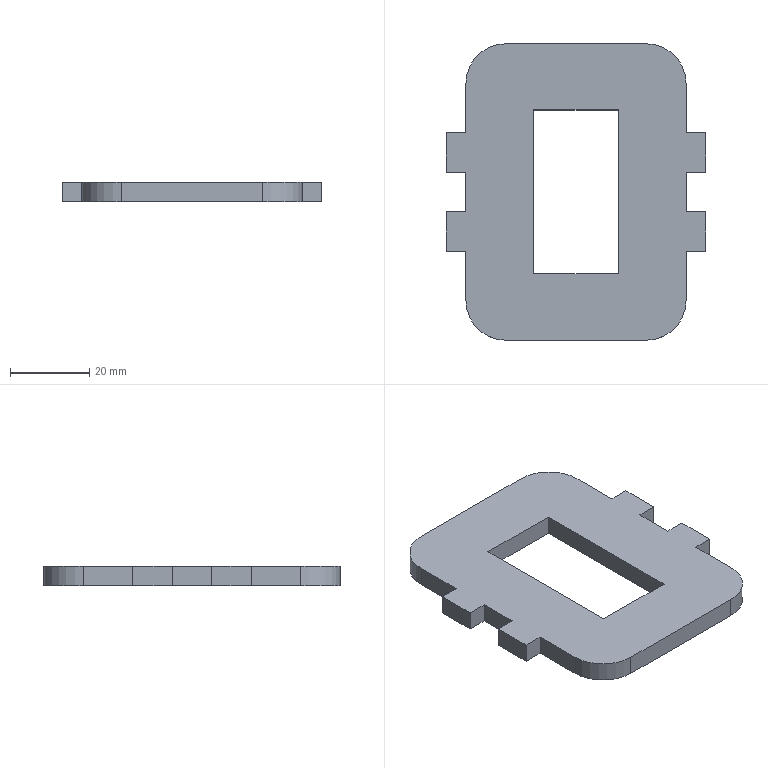Part | SolidWorks | features Extrusion 1, Fillet 1, ICE 1 | 1 solid | 30 faces | box 65.7 x 75 x 5 mm | volume 16997 mm3 | plane 26 | cylinder 4 | commonest cylinder face diameters 20 x4
STEP:
#1=CARTESIAN_POINT('',(32.85,-5.,0.));
#2=VERTEX_POINT('',#1);
#3=CARTESIAN_POINT('',(27.85,-5.,0.));
#4=VERTEX_POINT('',#3);
#5=CARTESIAN_POINT('',(0.,-5.,0.));
#6=DIRECTION('',(-1.,0.,0.));
#7=VECTOR('',#6,1000.);
#8=LINE('',#5,#7);
#9=EDGE_CURVE('',#2,#4,#8,.T.);
#10=ORIENTED_EDGE('',*,*,#9,.T.);
#11=CARTESIAN_POINT('',(27.85,-5.,5.));
#12=VERTEX_POINT('',#11);
#13=CARTESIAN_POINT('',(27.85,-5.,5.));
#14=DIRECTION('',(0.,0.,-1.));
#15=VECTOR('',#14,1000.);
#16=LINE('',#13,#15);
#17=EDGE_CURVE('',#12,#4,#16,.T.);
#18=ORIENTED_EDGE('',*,*,#17,.F.);
#19=CARTESIAN_POINT('',(32.85,-5.,5.));
#20=VERTEX_POINT('',#19);
#21=CARTESIAN_POINT('',(0.,-5.,5.));
#22=DIRECTION('',(-1.,0.,0.));
#23=VECTOR('',#22,1000.);
#24=LINE('',#21,#23);
#25=EDGE_CURVE('',#20,#12,#24,.T.);
#26=ORIENTED_EDGE('',*,*,#25,.F.);
#27=CARTESIAN_POINT('',(32.85,-5.,5.));
#28=DIRECTION('',(0.,0.,-1.));
#29=VECTOR('',#28,1000.);
#30=LINE('',#27,#29);
#31=EDGE_CURVE('',#20,#2,#30,.T.);
#32=ORIENTED_EDGE('',*,*,#31,.T.);
#33=EDGE_LOOP('',(#10,#18,#26,#32));
#34=FACE_OUTER_BOUND('',#33,.T.);
#35=CARTESIAN_POINT('',(0.,-5.,5.));
#36=DIRECTION('',(0.,-1.,0.));
#37=DIRECTION('',(0.,0.,-1.));
#38=AXIS2_PLACEMENT_3D('',#35,#36,#37);
#39=PLANE('',#38);
#40=ADVANCED_FACE('',(#34),#39,.F.);
#41=CARTESIAN_POINT('',(27.85,5.,0.));
#42=VERTEX_POINT('',#41);
#43=CARTESIAN_POINT('',(27.85,0.,0.));
#44=DIRECTION('',(0.,1.,0.));
#45=VECTOR('',#44,1000.);
#46=LINE('',#43,#45);
#47=EDGE_CURVE('',#4,#42,#46,.T.);
#48=ORIENTED_EDGE('',*,*,#47,.T.);
#49=CARTESIAN_POINT('',(27.85,5.,5.));
#50=VERTEX_POINT('',#49);
#51=CARTESIAN_POINT('',(27.85,5.,5.));
#52=DIRECTION('',(0.,0.,-1.));
#53=VECTOR('',#52,1000.);
#54=LINE('',#51,#53);
#55=EDGE_CURVE('',#50,#42,#54,.T.);
#56=ORIENTED_EDGE('',*,*,#55,.F.);
#57=CARTESIAN_POINT('',(27.85,0.,5.));
#58=DIRECTION('',(0.,1.,0.));
#59=VECTOR('',#58,1000.);
#60=LINE('',#57,#59);
#61=EDGE_CURVE('',#12,#50,#60,.T.);
#62=ORIENTED_EDGE('',*,*,#61,.F.);
#63=ORIENTED_EDGE('',*,*,#17,.T.);
#64=EDGE_LOOP('',(#48,#56,#62,#63));
#65=FACE_OUTER_BOUND('',#64,.T.);
#66=CARTESIAN_POINT('',(27.85,0.,5.));
#67=DIRECTION('',(-1.,0.,0.));
#68=DIRECTION('',(0.,0.,1.));
#69=AXIS2_PLACEMENT_3D('',#66,#67,#68);
#70=PLANE('',#69);
#71=ADVANCED_FACE('',(#65),#70,.F.);
#72=CARTESIAN_POINT('',(32.85,5.,0.));
#73=VERTEX_POINT('',#72);
#74=CARTESIAN_POINT('',(0.,5.,0.));
#75=DIRECTION('',(-1.,0.,0.));
#76=VECTOR('',#75,1000.);
#77=LINE('',#74,#76);
#78=EDGE_CURVE('',#73,#42,#77,.T.);
#79=ORIENTED_EDGE('',*,*,#78,.F.);
#80=CARTESIAN_POINT('',(32.85,5.,5.));
#81=VERTEX_POINT('',#80);
#82=CARTESIAN_POINT('',(32.85,5.,5.));
#83=DIRECTION('',(0.,0.,-1.));
#84=VECTOR('',#83,1000.);
#85=LINE('',#82,#84);
#86=EDGE_CURVE('',#81,#73,#85,.T.);
#87=ORIENTED_EDGE('',*,*,#86,.F.);
#88=CARTESIAN_POINT('',(0.,5.,5.));
#89=DIRECTION('',(-1.,0.,0.));
#90=VECTOR('',#89,1000.);
#91=LINE('',#88,#90);
#92=EDGE_CURVE('',#81,#50,#91,.T.);
#93=ORIENTED_EDGE('',*,*,#92,.T.);
#94=ORIENTED_EDGE('',*,*,#55,.T.);
#95=EDGE_LOOP('',(#79,#87,#93,#94));
#96=FACE_OUTER_BOUND('',#95,.T.);
#97=CARTESIAN_POINT('',(0.,5.,5.));
#98=DIRECTION('',(0.,-1.,0.));
#99=DIRECTION('',(0.,0.,-1.));
#100=AXIS2_PLACEMENT_3D('',#97,#98,#99);
#101=PLANE('',#100);
#102=ADVANCED_FACE('',(#96),#101,.T.);
#103=CARTESIAN_POINT('',(32.85,15.,0.));
#104=VERTEX_POINT('',#103);
#105=CARTESIAN_POINT('',(32.85,0.,0.));
#106=DIRECTION('',(0.,1.,0.));
#107=VECTOR('',#106,1000.);
#108=LINE('',#105,#107);
#109=EDGE_CURVE('',#73,#104,#108,.T.);
#110=ORIENTED_EDGE('',*,*,#109,.T.);
#111=CARTESIAN_POINT('',(32.85,15.,5.));
#112=VERTEX_POINT('',#111);
#113=CARTESIAN_POINT('',(32.85,15.,5.));
#114=DIRECTION('',(0.,0.,-1.));
#115=VECTOR('',#114,1000.);
#116=LINE('',#113,#115);
#117=EDGE_CURVE('',#112,#104,#116,.T.);
#118=ORIENTED_EDGE('',*,*,#117,.F.);
#119=CARTESIAN_POINT('',(32.85,0.,5.));
#120=DIRECTION('',(0.,1.,0.));
#121=VECTOR('',#120,1000.);
#122=LINE('',#119,#121);
#123=EDGE_CURVE('',#81,#112,#122,.T.);
#124=ORIENTED_EDGE('',*,*,#123,.F.);
#125=ORIENTED_EDGE('',*,*,#86,.T.);
#126=EDGE_LOOP('',(#110,#118,#124,#125));
#127=FACE_OUTER_BOUND('',#126,.T.);
#128=CARTESIAN_POINT('',(32.85,0.,5.));
#129=DIRECTION('',(-1.,0.,0.));
#130=DIRECTION('',(0.,0.,1.));
#131=AXIS2_PLACEMENT_3D('',#128,#129,#130);
#132=PLANE('',#131);
#133=ADVANCED_FACE('',(#127),#132,.F.);
#134=CARTESIAN_POINT('',(27.85,15.,0.));
#135=VERTEX_POINT('',#134);
#136=CARTESIAN_POINT('',(0.,15.,0.));
#137=DIRECTION('',(-1.,0.,0.));
#138=VECTOR('',#137,1000.);
#139=LINE('',#136,#138);
#140=EDGE_CURVE('',#104,#135,#139,.T.);
#141=ORIENTED_EDGE('',*,*,#140,.T.);
#142=CARTESIAN_POINT('',(27.85,15.,5.));
#143=VERTEX_POINT('',#142);
#144=CARTESIAN_POINT('',(27.85,15.,5.));
#145=DIRECTION('',(0.,0.,-1.));
#146=VECTOR('',#145,1000.);
#147=LINE('',#144,#146);
#148=EDGE_CURVE('',#143,#135,#147,.T.);
#149=ORIENTED_EDGE('',*,*,#148,.F.);
#150=CARTESIAN_POINT('',(0.,15.,5.));
#151=DIRECTION('',(-1.,0.,0.));
#152=VECTOR('',#151,1000.);
#153=LINE('',#150,#152);
#154=EDGE_CURVE('',#112,#143,#153,.T.);
#155=ORIENTED_EDGE('',*,*,#154,.F.);
#156=ORIENTED_EDGE('',*,*,#117,.T.);
#157=EDGE_LOOP('',(#141,#149,#155,#156));
#158=FACE_OUTER_BOUND('',#157,.T.);
#159=CARTESIAN_POINT('',(0.,15.,5.));
#160=DIRECTION('',(0.,-1.,0.));
#161=DIRECTION('',(0.,0.,-1.));
#162=AXIS2_PLACEMENT_3D('',#159,#160,#161);
#163=PLANE('',#162);
#164=ADVANCED_FACE('',(#158),#163,.F.);
#165=CARTESIAN_POINT('',(27.85,27.5,0.));
#166=VERTEX_POINT('',#165);
#167=CARTESIAN_POINT('',(27.85,0.,0.));
#168=DIRECTION('',(0.,1.,0.));
#169=VECTOR('',#168,1000.);
#170=LINE('',#167,#169);
#171=EDGE_CURVE('',#135,#166,#170,.T.);
#172=ORIENTED_EDGE('',*,*,#171,.T.);
#173=CARTESIAN_POINT('',(27.85,27.5,5.));
#174=VERTEX_POINT('',#173);
#175=CARTESIAN_POINT('',(27.85,27.5,5.));
#176=DIRECTION('',(0.,0.,1.));
#177=VECTOR('',#176,1000.);
#178=LINE('',#175,#177);
#179=EDGE_CURVE('',#166,#174,#178,.T.);
#180=ORIENTED_EDGE('',*,*,#179,.T.);
#181=CARTESIAN_POINT('',(27.85,0.,5.));
#182=DIRECTION('',(0.,1.,0.));
#183=VECTOR('',#182,1000.);
#184=LINE('',#181,#183);
#185=EDGE_CURVE('',#143,#174,#184,.T.);
#186=ORIENTED_EDGE('',*,*,#185,.F.);
#187=ORIENTED_EDGE('',*,*,#148,.T.);
#188=EDGE_LOOP('',(#172,#180,#186,#187));
#189=FACE_OUTER_BOUND('',#188,.T.);
#190=CARTESIAN_POINT('',(27.85,0.,5.));
#191=DIRECTION('',(-1.,0.,0.));
#192=DIRECTION('',(0.,0.,1.));
#193=AXIS2_PLACEMENT_3D('',#190,#191,#192);
#194=PLANE('',#193);
#195=ADVANCED_FACE('',(#189),#194,.F.);
#196=CARTESIAN_POINT('',(-17.85,37.5,0.));
#197=VERTEX_POINT('',#196);
#198=CARTESIAN_POINT('',(17.85,37.5,0.));
#199=VERTEX_POINT('',#198);
#200=CARTESIAN_POINT('',(0.,37.5,0.));
#201=DIRECTION('',(1.,0.,0.));
#202=VECTOR('',#201,1000.);
#203=LINE('',#200,#202);
#204=EDGE_CURVE('',#197,#199,#203,.T.);
#205=ORIENTED_EDGE('',*,*,#204,.F.);
#206=CARTESIAN_POINT('',(-17.85,37.5,5.));
#207=VERTEX_POINT('',#206);
#208=CARTESIAN_POINT('',(-17.85,37.5,5.));
#209=DIRECTION('',(0.,0.,1.));
#210=VECTOR('',#209,1000.);
#211=LINE('',#208,#210);
#212=EDGE_CURVE('',#197,#207,#211,.T.);
#213=ORIENTED_EDGE('',*,*,#212,.T.);
#214=CARTESIAN_POINT('',(17.85,37.5,5.));
#215=VERTEX_POINT('',#214);
#216=CARTESIAN_POINT('',(0.,37.5,5.));
#217=DIRECTION('',(1.,0.,0.));
#218=VECTOR('',#217,1000.);
#219=LINE('',#216,#218);
#220=EDGE_CURVE('',#207,#215,#219,.T.);
#221=ORIENTED_EDGE('',*,*,#220,.T.);
#222=CARTESIAN_POINT('',(17.85,37.5,0.));
#223=DIRECTION('',(0.,0.,-1.));
#224=VECTOR('',#223,1000.);
#225=LINE('',#222,#224);
#226=EDGE_CURVE('',#215,#199,#225,.T.);
#227=ORIENTED_EDGE('',*,*,#226,.T.);
#228=EDGE_LOOP('',(#205,#213,#221,#227));
#229=FACE_OUTER_BOUND('',#228,.T.);
#230=CARTESIAN_POINT('',(0.,37.5,5.));
#231=DIRECTION('',(0.,1.,0.));
#232=DIRECTION('',(-1.,0.,0.));
#233=AXIS2_PLACEMENT_3D('',#230,#231,#232);
#234=PLANE('',#233);
#235=ADVANCED_FACE('',(#229),#234,.T.);
#236=CARTESIAN_POINT('',(-27.85,15.,5.));
#237=VERTEX_POINT('',#236);
#238=CARTESIAN_POINT('',(-27.85,27.5,5.));
#239=VERTEX_POINT('',#238);
#240=CARTESIAN_POINT('',(-27.85,0.,5.));
#241=DIRECTION('',(0.,1.,0.));
#242=VECTOR('',#241,1000.);
#243=LINE('',#240,#242);
#244=EDGE_CURVE('',#237,#239,#243,.T.);
#245=ORIENTED_EDGE('',*,*,#244,.T.);
#246=CARTESIAN_POINT('',(-27.85,27.5,0.));
#247=VERTEX_POINT('',#246);
#248=CARTESIAN_POINT('',(-27.85,27.5,5.));
#249=DIRECTION('',(0.,0.,-1.));
#250=VECTOR('',#249,1000.);
#251=LINE('',#248,#250);
#252=EDGE_CURVE('',#239,#247,#251,.T.);
#253=ORIENTED_EDGE('',*,*,#252,.T.);
#254=CARTESIAN_POINT('',(-27.85,15.,0.));
#255=VERTEX_POINT('',#254);
#256=CARTESIAN_POINT('',(-27.85,0.,0.));
#257=DIRECTION('',(0.,1.,0.));
#258=VECTOR('',#257,1000.);
#259=LINE('',#256,#258);
#260=EDGE_CURVE('',#255,#247,#259,.T.);
#261=ORIENTED_EDGE('',*,*,#260,.F.);
#262=CARTESIAN_POINT('',(-27.85,15.,5.));
#263=DIRECTION('',(0.,0.,-1.));
#264=VECTOR('',#263,1000.);
#265=LINE('',#262,#264);
#266=EDGE_CURVE('',#237,#255,#265,.T.);
#267=ORIENTED_EDGE('',*,*,#266,.F.);
#268=EDGE_LOOP('',(#245,#253,#261,#267));
#269=FACE_OUTER_BOUND('',#268,.T.);
#270=CARTESIAN_POINT('',(-27.85,0.,5.));
#271=DIRECTION('',(-1.,0.,0.));
#272=DIRECTION('',(0.,-1.,0.));
#273=AXIS2_PLACEMENT_3D('',#270,#271,#272);
#274=PLANE('',#273);
#275=ADVANCED_FACE('',(#269),#274,.T.);
#276=CARTESIAN_POINT('',(-32.85,15.,0.));
#277=VERTEX_POINT('',#276);
#278=CARTESIAN_POINT('',(0.,15.,0.));
#279=DIRECTION('',(1.,0.,0.));
#280=VECTOR('',#279,1000.);
#281=LINE('',#278,#280);
#282=EDGE_CURVE('',#277,#255,#281,.T.);
#283=ORIENTED_EDGE('',*,*,#282,.F.);
#284=CARTESIAN_POINT('',(-32.85,15.,5.));
#285=VERTEX_POINT('',#284);
#286=CARTESIAN_POINT('',(-32.85,15.,5.));
#287=DIRECTION('',(0.,0.,-1.));
#288=VECTOR('',#287,1000.);
#289=LINE('',#286,#288);
#290=EDGE_CURVE('',#285,#277,#289,.T.);
#291=ORIENTED_EDGE('',*,*,#290,.F.);
#292=CARTESIAN_POINT('',(0.,15.,5.));
#293=DIRECTION('',(1.,0.,0.));
#294=VECTOR('',#293,1000.);
#295=LINE('',#292,#294);
#296=EDGE_CURVE('',#285,#237,#295,.T.);
#297=ORIENTED_EDGE('',*,*,#296,.T.);
#298=ORIENTED_EDGE('',*,*,#266,.T.);
#299=EDGE_LOOP('',(#283,#291,#297,#298));
#300=FACE_OUTER_BOUND('',#299,.T.);
#301=CARTESIAN_POINT('',(0.,15.,5.));
#302=DIRECTION('',(0.,1.,0.));
#303=DIRECTION('',(0.,0.,1.));
#304=AXIS2_PLACEMENT_3D('',#301,#302,#303);
#305=PLANE('',#304);
#306=ADVANCED_FACE('',(#300),#305,.T.);
#307=CARTESIAN_POINT('',(-32.85,5.,0.));
#308=VERTEX_POINT('',#307);
#309=CARTESIAN_POINT('',(-32.85,0.,0.));
#310=DIRECTION('',(0.,1.,0.));
#311=VECTOR('',#310,1000.);
#312=LINE('',#309,#311);
#313=EDGE_CURVE('',#308,#277,#312,.T.);
#314=ORIENTED_EDGE('',*,*,#313,.F.);
#315=CARTESIAN_POINT('',(-32.85,5.,5.));
#316=VERTEX_POINT('',#315);
#317=CARTESIAN_POINT('',(-32.85,5.,5.));
#318=DIRECTION('',(0.,0.,-1.));
#319=VECTOR('',#318,1000.);
#320=LINE('',#317,#319);
#321=EDGE_CURVE('',#316,#308,#320,.T.);
#322=ORIENTED_EDGE('',*,*,#321,.F.);
#323=CARTESIAN_POINT('',(-32.85,0.,5.));
#324=DIRECTION('',(0.,1.,0.));
#325=VECTOR('',#324,1000.);
#326=LINE('',#323,#325);
#327=EDGE_CURVE('',#316,#285,#326,.T.);
#328=ORIENTED_EDGE('',*,*,#327,.T.);
#329=ORIENTED_EDGE('',*,*,#290,.T.);
#330=EDGE_LOOP('',(#314,#322,#328,#329));
#331=FACE_OUTER_BOUND('',#330,.T.);
#332=CARTESIAN_POINT('',(-32.85,0.,5.));
#333=DIRECTION('',(-1.,0.,0.));
#334=DIRECTION('',(0.,0.,1.));
#335=AXIS2_PLACEMENT_3D('',#332,#333,#334);
#336=PLANE('',#335);
#337=ADVANCED_FACE('',(#331),#336,.T.);
#338=CARTESIAN_POINT('',(-27.85,5.,0.));
#339=VERTEX_POINT('',#338);
#340=CARTESIAN_POINT('',(0.,5.,0.));
#341=DIRECTION('',(1.,0.,0.));
#342=VECTOR('',#341,1000.);
#343=LINE('',#340,#342);
#344=EDGE_CURVE('',#308,#339,#343,.T.);
#345=ORIENTED_EDGE('',*,*,#344,.T.);
#346=CARTESIAN_POINT('',(-27.85,5.,5.));
#347=VERTEX_POINT('',#346);
#348=CARTESIAN_POINT('',(-27.85,5.,5.));
#349=DIRECTION('',(0.,0.,-1.));
#350=VECTOR('',#349,1000.);
#351=LINE('',#348,#350);
#352=EDGE_CURVE('',#347,#339,#351,.T.);
#353=ORIENTED_EDGE('',*,*,#352,.F.);
#354=CARTESIAN_POINT('',(0.,5.,5.));
#355=DIRECTION('',(1.,0.,0.));
#356=VECTOR('',#355,1000.);
#357=LINE('',#354,#356);
#358=EDGE_CURVE('',#316,#347,#357,.T.);
#359=ORIENTED_EDGE('',*,*,#358,.F.);
#360=ORIENTED_EDGE('',*,*,#321,.T.);
#361=EDGE_LOOP('',(#345,#353,#359,#360));
#362=FACE_OUTER_BOUND('',#361,.T.);
#363=CARTESIAN_POINT('',(0.,5.,5.));
#364=DIRECTION('',(0.,1.,0.));
#365=DIRECTION('',(0.,0.,1.));
#366=AXIS2_PLACEMENT_3D('',#363,#364,#365);
#367=PLANE('',#366);
#368=ADVANCED_FACE('',(#362),#367,.F.);
#369=CARTESIAN_POINT('',(-27.85,-5.,0.));
#370=VERTEX_POINT('',#369);
#371=CARTESIAN_POINT('',(-27.85,0.,0.));
#372=DIRECTION('',(0.,1.,0.));
#373=VECTOR('',#372,1000.);
#374=LINE('',#371,#373);
#375=EDGE_CURVE('',#370,#339,#374,.T.);
#376=ORIENTED_EDGE('',*,*,#375,.F.);
#377=CARTESIAN_POINT('',(-27.85,-5.,5.));
#378=VERTEX_POINT('',#377);
#379=CARTESIAN_POINT('',(-27.85,-5.,5.));
#380=DIRECTION('',(0.,0.,-1.));
#381=VECTOR('',#380,1000.);
#382=LINE('',#379,#381);
#383=EDGE_CURVE('',#378,#370,#382,.T.);
#384=ORIENTED_EDGE('',*,*,#383,.F.);
#385=CARTESIAN_POINT('',(-27.85,0.,5.));
#386=DIRECTION('',(0.,1.,0.));
#387=VECTOR('',#386,1000.);
#388=LINE('',#385,#387);
#389=EDGE_CURVE('',#378,#347,#388,.T.);
#390=ORIENTED_EDGE('',*,*,#389,.T.);
#391=ORIENTED_EDGE('',*,*,#352,.T.);
#392=EDGE_LOOP('',(#376,#384,#390,#391));
#393=FACE_OUTER_BOUND('',#392,.T.);
#394=CARTESIAN_POINT('',(-27.85,0.,5.));
#395=DIRECTION('',(-1.,0.,0.));
#396=DIRECTION('',(0.,0.,1.));
#397=AXIS2_PLACEMENT_3D('',#394,#395,#396);
#398=PLANE('',#397);
#399=ADVANCED_FACE('',(#393),#398,.T.);
#400=CARTESIAN_POINT('',(-32.85,-5.,0.));
#401=VERTEX_POINT('',#400);
#402=CARTESIAN_POINT('',(0.,-5.,0.));
#403=DIRECTION('',(1.,0.,0.));
#404=VECTOR('',#403,1000.);
#405=LINE('',#402,#404);
#406=EDGE_CURVE('',#401,#370,#405,.T.);
#407=ORIENTED_EDGE('',*,*,#406,.F.);
#408=CARTESIAN_POINT('',(-32.85,-5.,5.));
#409=VERTEX_POINT('',#408);
#410=CARTESIAN_POINT('',(-32.85,-5.,5.));
#411=DIRECTION('',(0.,0.,-1.));
#412=VECTOR('',#411,1000.);
#413=LINE('',#410,#412);
#414=EDGE_CURVE('',#409,#401,#413,.T.);
#415=ORIENTED_EDGE('',*,*,#414,.F.);
#416=CARTESIAN_POINT('',(0.,-5.,5.));
#417=DIRECTION('',(1.,0.,0.));
#418=VECTOR('',#417,1000.);
#419=LINE('',#416,#418);
#420=EDGE_CURVE('',#409,#378,#419,.T.);
#421=ORIENTED_EDGE('',*,*,#420,.T.);
#422=ORIENTED_EDGE('',*,*,#383,.T.);
#423=EDGE_LOOP('',(#407,#415,#421,#422));
#424=FACE_OUTER_BOUND('',#423,.T.);
#425=CARTESIAN_POINT('',(0.,-5.,5.));
#426=DIRECTION('',(0.,1.,0.));
#427=DIRECTION('',(0.,0.,1.));
#428=AXIS2_PLACEMENT_3D('',#425,#426,#427);
#429=PLANE('',#428);
#430=ADVANCED_FACE('',(#424),#429,.T.);
#431=CARTESIAN_POINT('',(-32.85,-15.,0.));
#432=VERTEX_POINT('',#431);
#433=CARTESIAN_POINT('',(-32.85,0.,0.));
#434=DIRECTION('',(0.,1.,0.));
#435=VECTOR('',#434,1000.);
#436=LINE('',#433,#435);
#437=EDGE_CURVE('',#432,#401,#436,.T.);
#438=ORIENTED_EDGE('',*,*,#437,.F.);
#439=CARTESIAN_POINT('',(-32.85,-15.,5.));
#440=VERTEX_POINT('',#439);
#441=CARTESIAN_POINT('',(-32.85,-15.,5.));
#442=DIRECTION('',(0.,0.,-1.));
#443=VECTOR('',#442,1000.);
#444=LINE('',#441,#443);
#445=EDGE_CURVE('',#440,#432,#444,.T.);
#446=ORIENTED_EDGE('',*,*,#445,.F.);
#447=CARTESIAN_POINT('',(-32.85,0.,5.));
#448=DIRECTION('',(0.,1.,0.));
#449=VECTOR('',#448,1000.);
#450=LINE('',#447,#449);
#451=EDGE_CURVE('',#440,#409,#450,.T.);
#452=ORIENTED_EDGE('',*,*,#451,.T.);
#453=ORIENTED_EDGE('',*,*,#414,.T.);
#454=EDGE_LOOP('',(#438,#446,#452,#453));
#455=FACE_OUTER_BOUND('',#454,.T.);
#456=CARTESIAN_POINT('',(-32.85,0.,5.));
#457=DIRECTION('',(-1.,0.,0.));
#458=DIRECTION('',(0.,0.,1.));
#459=AXIS2_PLACEMENT_3D('',#456,#457,#458);
#460=PLANE('',#459);
#461=ADVANCED_FACE('',(#455),#460,.T.);
#462=CARTESIAN_POINT('',(-27.85,-15.,0.));
#463=VERTEX_POINT('',#462);
#464=CARTESIAN_POINT('',(0.,-15.,0.));
#465=DIRECTION('',(1.,0.,0.));
#466=VECTOR('',#465,1000.);
#467=LINE('',#464,#466);
#468=EDGE_CURVE('',#432,#463,#467,.T.);
#469=ORIENTED_EDGE('',*,*,#468,.T.);
#470=CARTESIAN_POINT('',(-27.85,-15.,5.));
#471=VERTEX_POINT('',#470);
#472=CARTESIAN_POINT('',(-27.85,-15.,5.));
#473=DIRECTION('',(0.,0.,-1.));
#474=VECTOR('',#473,1000.);
#475=LINE('',#472,#474);
#476=EDGE_CURVE('',#471,#463,#475,.T.);
#477=ORIENTED_EDGE('',*,*,#476,.F.);
#478=CARTESIAN_POINT('',(0.,-15.,5.));
#479=DIRECTION('',(1.,0.,0.));
#480=VECTOR('',#479,1000.);
#481=LINE('',#478,#480);
#482=EDGE_CURVE('',#440,#471,#481,.T.);
#483=ORIENTED_EDGE('',*,*,#482,.F.);
#484=ORIENTED_EDGE('',*,*,#445,.T.);
#485=EDGE_LOOP('',(#469,#477,#483,#484));
#486=FACE_OUTER_BOUND('',#485,.T.);
#487=CARTESIAN_POINT('',(0.,-15.,5.));
#488=DIRECTION('',(0.,1.,0.));
#489=DIRECTION('',(0.,0.,1.));
#490=AXIS2_PLACEMENT_3D('',#487,#488,#489);
#491=PLANE('',#490);
#492=ADVANCED_FACE('',(#486),#491,.F.);
#493=CARTESIAN_POINT('',(-27.85,-27.5,0.));
#494=VERTEX_POINT('',#493);
#495=CARTESIAN_POINT('',(-27.85,0.,0.));
#496=DIRECTION('',(0.,1.,0.));
#497=VECTOR('',#496,1000.);
#498=LINE('',#495,#497);
#499=EDGE_CURVE('',#494,#463,#498,.T.);
#500=ORIENTED_EDGE('',*,*,#499,.F.);
#501=CARTESIAN_POINT('',(-27.85,-27.5,5.));
#502=VERTEX_POINT('',#501);
#503=CARTESIAN_POINT('',(-27.85,-27.5,5.));
#504=DIRECTION('',(0.,0.,1.));
#505=VECTOR('',#504,1000.);
#506=LINE('',#503,#505);
#507=EDGE_CURVE('',#494,#502,#506,.T.);
#508=ORIENTED_EDGE('',*,*,#507,.T.);
#509=CARTESIAN_POINT('',(-27.85,0.,5.));
#510=DIRECTION('',(0.,1.,0.));
#511=VECTOR('',#510,1000.);
#512=LINE('',#509,#511);
#513=EDGE_CURVE('',#502,#471,#512,.T.);
#514=ORIENTED_EDGE('',*,*,#513,.T.);
#515=ORIENTED_EDGE('',*,*,#476,.T.);
#516=EDGE_LOOP('',(#500,#508,#514,#515));
#517=FACE_OUTER_BOUND('',#516,.T.);
#518=CARTESIAN_POINT('',(-27.85,0.,5.));
#519=DIRECTION('',(-1.,0.,0.));
#520=DIRECTION('',(0.,0.,1.));
#521=AXIS2_PLACEMENT_3D('',#518,#519,#520);
#522=PLANE('',#521);
#523=ADVANCED_FACE('',(#517),#522,.T.);
#524=CARTESIAN_POINT('',(-17.85,-37.5,0.));
#525=VERTEX_POINT('',#524);
#526=CARTESIAN_POINT('',(17.85,-37.5,0.));
#527=VERTEX_POINT('',#526);
#528=CARTESIAN_POINT('',(0.,-37.5,0.));
#529=DIRECTION('',(1.,0.,0.));
#530=VECTOR('',#529,1000.);
#531=LINE('',#528,#530);
#532=EDGE_CURVE('',#525,#527,#531,.T.);
#533=ORIENTED_EDGE('',*,*,#532,.T.);
#534=CARTESIAN_POINT('',(17.85,-37.5,5.));
#535=VERTEX_POINT('',#534);
#536=CARTESIAN_POINT('',(17.85,-37.5,5.));
#537=DIRECTION('',(0.,0.,1.));
#538=VECTOR('',#537,1000.);
#539=LINE('',#536,#538);
#540=EDGE_CURVE('',#527,#535,#539,.T.);
#541=ORIENTED_EDGE('',*,*,#540,.T.);
#542=CARTESIAN_POINT('',(-17.85,-37.5,5.));
#543=VERTEX_POINT('',#542);
#544=CARTESIAN_POINT('',(0.,-37.5,5.));
#545=DIRECTION('',(1.,0.,0.));
#546=VECTOR('',#545,1000.);
#547=LINE('',#544,#546);
#548=EDGE_CURVE('',#543,#535,#547,.T.);
#549=ORIENTED_EDGE('',*,*,#548,.F.);
#550=CARTESIAN_POINT('',(-17.85,-37.5,0.));
#551=DIRECTION('',(0.,0.,-1.));
#552=VECTOR('',#551,1000.);
#553=LINE('',#550,#552);
#554=EDGE_CURVE('',#543,#525,#553,.T.);
#555=ORIENTED_EDGE('',*,*,#554,.T.);
#556=EDGE_LOOP('',(#533,#541,#549,#555));
#557=FACE_OUTER_BOUND('',#556,.T.);
#558=CARTESIAN_POINT('',(0.,-37.5,5.));
#559=DIRECTION('',(0.,1.,0.));
#560=DIRECTION('',(0.,0.,1.));
#561=AXIS2_PLACEMENT_3D('',#558,#559,#560);
#562=PLANE('',#561);
#563=ADVANCED_FACE('',(#557),#562,.F.);
#564=CARTESIAN_POINT('',(27.85,-27.5,5.));
#565=VERTEX_POINT('',#564);
#566=CARTESIAN_POINT('',(27.85,-15.,5.));
#567=VERTEX_POINT('',#566);
#568=CARTESIAN_POINT('',(27.85,0.,5.));
#569=DIRECTION('',(0.,1.,0.));
#570=VECTOR('',#569,1000.);
#571=LINE('',#568,#570);
#572=EDGE_CURVE('',#565,#567,#571,.T.);
#573=ORIENTED_EDGE('',*,*,#572,.F.);
#574=CARTESIAN_POINT('',(27.85,-27.5,0.));
#575=VERTEX_POINT('',#574);
#576=CARTESIAN_POINT('',(27.85,-27.5,5.));
#577=DIRECTION('',(0.,0.,-1.));
#578=VECTOR('',#577,1000.);
#579=LINE('',#576,#578);
#580=EDGE_CURVE('',#565,#575,#579,.T.);
#581=ORIENTED_EDGE('',*,*,#580,.T.);
#582=CARTESIAN_POINT('',(27.85,-15.,0.));
#583=VERTEX_POINT('',#582);
#584=CARTESIAN_POINT('',(27.85,0.,0.));
#585=DIRECTION('',(0.,1.,0.));
#586=VECTOR('',#585,1000.);
#587=LINE('',#584,#586);
#588=EDGE_CURVE('',#575,#583,#587,.T.);
#589=ORIENTED_EDGE('',*,*,#588,.T.);
#590=CARTESIAN_POINT('',(27.85,-15.,5.));
#591=DIRECTION('',(0.,0.,-1.));
#592=VECTOR('',#591,1000.);
#593=LINE('',#590,#592);
#594=EDGE_CURVE('',#567,#583,#593,.T.);
#595=ORIENTED_EDGE('',*,*,#594,.F.);
#596=EDGE_LOOP('',(#573,#581,#589,#595));
#597=FACE_OUTER_BOUND('',#596,.T.);
#598=CARTESIAN_POINT('',(27.85,0.,5.));
#599=DIRECTION('',(-1.,0.,0.));
#600=DIRECTION('',(0.,-1.,0.));
#601=AXIS2_PLACEMENT_3D('',#598,#599,#600);
#602=PLANE('',#601);
#603=ADVANCED_FACE('',(#597),#602,.F.);
#604=CARTESIAN_POINT('',(32.85,-15.,0.));
#605=VERTEX_POINT('',#604);
#606=CARTESIAN_POINT('',(0.,-15.,0.));
#607=DIRECTION('',(-1.,0.,0.));
#608=VECTOR('',#607,1000.);
#609=LINE('',#606,#608);
#610=EDGE_CURVE('',#605,#583,#609,.T.);
#611=ORIENTED_EDGE('',*,*,#610,.F.);
#612=CARTESIAN_POINT('',(32.85,-15.,5.));
#613=VERTEX_POINT('',#612);
#614=CARTESIAN_POINT('',(32.85,-15.,5.));
#615=DIRECTION('',(0.,0.,-1.));
#616=VECTOR('',#615,1000.);
#617=LINE('',#614,#616);
#618=EDGE_CURVE('',#613,#605,#617,.T.);
#619=ORIENTED_EDGE('',*,*,#618,.F.);
#620=CARTESIAN_POINT('',(0.,-15.,5.));
#621=DIRECTION('',(-1.,0.,0.));
#622=VECTOR('',#621,1000.);
#623=LINE('',#620,#622);
#624=EDGE_CURVE('',#613,#567,#623,.T.);
#625=ORIENTED_EDGE('',*,*,#624,.T.);
#626=ORIENTED_EDGE('',*,*,#594,.T.);
#627=EDGE_LOOP('',(#611,#619,#625,#626));
#628=FACE_OUTER_BOUND('',#627,.T.);
#629=CARTESIAN_POINT('',(0.,-15.,5.));
#630=DIRECTION('',(0.,-1.,0.));
#631=DIRECTION('',(0.,0.,-1.));
#632=AXIS2_PLACEMENT_3D('',#629,#630,#631);
#633=PLANE('',#632);
#634=ADVANCED_FACE('',(#628),#633,.T.);
#635=CARTESIAN_POINT('',(32.85,0.,0.));
#636=DIRECTION('',(0.,1.,0.));
#637=VECTOR('',#636,1000.);
#638=LINE('',#635,#637);
#639=EDGE_CURVE('',#605,#2,#638,.T.);
#640=ORIENTED_EDGE('',*,*,#639,.T.);
#641=ORIENTED_EDGE('',*,*,#31,.F.);
#642=CARTESIAN_POINT('',(32.85,0.,5.));
#643=DIRECTION('',(0.,1.,0.));
#644=VECTOR('',#643,1000.);
#645=LINE('',#642,#644);
#646=EDGE_CURVE('',#613,#20,#645,.T.);
#647=ORIENTED_EDGE('',*,*,#646,.F.);
#648=ORIENTED_EDGE('',*,*,#618,.T.);
#649=EDGE_LOOP('',(#640,#641,#647,#648));
#650=FACE_OUTER_BOUND('',#649,.T.);
#651=CARTESIAN_POINT('',(32.85,0.,5.));
#652=DIRECTION('',(-1.,0.,0.));
#653=DIRECTION('',(0.,0.,1.));
#654=AXIS2_PLACEMENT_3D('',#651,#652,#653);
#655=PLANE('',#654);
#656=ADVANCED_FACE('',(#650),#655,.F.);
#657=CARTESIAN_POINT('',(10.75,-20.75,5.));
#658=VERTEX_POINT('',#657);
#659=CARTESIAN_POINT('',(10.75,20.75,5.));
#660=VERTEX_POINT('',#659);
#661=CARTESIAN_POINT('',(10.75,-20.75,5.));
#662=DIRECTION('',(0.,1.,0.));
#663=VECTOR('',#662,1000.);
#664=LINE('',#661,#663);
#665=EDGE_CURVE('',#658,#660,#664,.T.);
#666=ORIENTED_EDGE('',*,*,#665,.F.);
#667=CARTESIAN_POINT('',(-10.75,-20.75,5.));
#668=VERTEX_POINT('',#667);
#669=CARTESIAN_POINT('',(-10.75,-20.75,5.));
#670=DIRECTION('',(1.,0.,0.));
#671=VECTOR('',#670,1000.);
#672=LINE('',#669,#671);
#673=EDGE_CURVE('',#668,#658,#672,.T.);
#674=ORIENTED_EDGE('',*,*,#673,.F.);
#675=CARTESIAN_POINT('',(-10.75,20.75,5.));
#676=VERTEX_POINT('',#675);
#677=CARTESIAN_POINT('',(-10.75,-20.75,5.));
#678=DIRECTION('',(0.,-1.,0.));
#679=VECTOR('',#678,1000.);
#680=LINE('',#677,#679);
#681=EDGE_CURVE('',#676,#668,#680,.T.);
#682=ORIENTED_EDGE('',*,*,#681,.F.);
#683=CARTESIAN_POINT('',(-10.75,20.75,5.));
#684=DIRECTION('',(-1.,0.,0.));
#685=VECTOR('',#684,1000.);
#686=LINE('',#683,#685);
#687=EDGE_CURVE('',#660,#676,#686,.T.);
#688=ORIENTED_EDGE('',*,*,#687,.F.);
#689=EDGE_LOOP('',(#666,#674,#682,#688));
#690=FACE_BOUND('',#689,.T.);
#691=ORIENTED_EDGE('',*,*,#548,.T.);
#692=CARTESIAN_POINT('',(17.85,-27.5,5.));
#693=DIRECTION('',(0.,0.,1.));
#694=DIRECTION('',(1.,0.,0.));
#695=AXIS2_PLACEMENT_3D('',#692,#693,#694);
#696=CIRCLE('',#695,10.);
#697=EDGE_CURVE('',#535,#565,#696,.T.);
#698=ORIENTED_EDGE('',*,*,#697,.T.);
#699=ORIENTED_EDGE('',*,*,#572,.T.);
#700=ORIENTED_EDGE('',*,*,#624,.F.);
#701=ORIENTED_EDGE('',*,*,#646,.T.);
#702=ORIENTED_EDGE('',*,*,#25,.T.);
#703=ORIENTED_EDGE('',*,*,#61,.T.);
#704=ORIENTED_EDGE('',*,*,#92,.F.);
#705=ORIENTED_EDGE('',*,*,#123,.T.);
#706=ORIENTED_EDGE('',*,*,#154,.T.);
#707=ORIENTED_EDGE('',*,*,#185,.T.);
#708=CARTESIAN_POINT('',(17.85,27.5,5.));
#709=DIRECTION('',(0.,0.,1.));
#710=DIRECTION('',(1.,0.,0.));
#711=AXIS2_PLACEMENT_3D('',#708,#709,#710);
#712=CIRCLE('',#711,10.);
#713=EDGE_CURVE('',#174,#215,#712,.T.);
#714=ORIENTED_EDGE('',*,*,#713,.T.);
#715=ORIENTED_EDGE('',*,*,#220,.F.);
#716=CARTESIAN_POINT('',(-17.85,27.5,5.));
#717=DIRECTION('',(0.,0.,1.));
#718=DIRECTION('',(1.,0.,0.));
#719=AXIS2_PLACEMENT_3D('',#716,#717,#718);
#720=CIRCLE('',#719,10.);
#721=EDGE_CURVE('',#207,#239,#720,.T.);
#722=ORIENTED_EDGE('',*,*,#721,.T.);
#723=ORIENTED_EDGE('',*,*,#244,.F.);
#724=ORIENTED_EDGE('',*,*,#296,.F.);
#725=ORIENTED_EDGE('',*,*,#327,.F.);
#726=ORIENTED_EDGE('',*,*,#358,.T.);
#727=ORIENTED_EDGE('',*,*,#389,.F.);
#728=ORIENTED_EDGE('',*,*,#420,.F.);
#729=ORIENTED_EDGE('',*,*,#451,.F.);
#730=ORIENTED_EDGE('',*,*,#482,.T.);
#731=ORIENTED_EDGE('',*,*,#513,.F.);
#732=CARTESIAN_POINT('',(-17.85,-27.5,5.));
#733=DIRECTION('',(0.,0.,1.));
#734=DIRECTION('',(1.,0.,0.));
#735=AXIS2_PLACEMENT_3D('',#732,#733,#734);
#736=CIRCLE('',#735,10.);
#737=EDGE_CURVE('',#502,#543,#736,.T.);
#738=ORIENTED_EDGE('',*,*,#737,.T.);
#739=EDGE_LOOP('',(#691,#698,#699,#700,#701,#702,#703,#704,#705,#706,#707,#714,#715,#722,#723,#724,#725,#726,#727,#728,#729,#730,#731,#738));
#740=FACE_OUTER_BOUND('',#739,.T.);
#741=CARTESIAN_POINT('',(0.,0.,5.));
#742=DIRECTION('',(0.,0.,1.));
#743=DIRECTION('',(1.,0.,0.));
#744=AXIS2_PLACEMENT_3D('',#741,#742,#743);
#745=PLANE('',#744);
#746=ADVANCED_FACE('',(#690,#740),#745,.T.);
#747=CARTESIAN_POINT('',(-10.75,-20.75,0.));
#748=VERTEX_POINT('',#747);
#749=CARTESIAN_POINT('',(10.75,-20.75,0.));
#750=VERTEX_POINT('',#749);
#751=CARTESIAN_POINT('',(-10.75,-20.75,0.));
#752=DIRECTION('',(1.,0.,0.));
#753=VECTOR('',#752,1000.);
#754=LINE('',#751,#753);
#755=EDGE_CURVE('',#748,#750,#754,.T.);
#756=ORIENTED_EDGE('',*,*,#755,.T.);
#757=CARTESIAN_POINT('',(10.75,20.75,0.));
#758=VERTEX_POINT('',#757);
#759=CARTESIAN_POINT('',(10.75,-20.75,0.));
#760=DIRECTION('',(0.,1.,0.));
#761=VECTOR('',#760,1000.);
#762=LINE('',#759,#761);
#763=EDGE_CURVE('',#750,#758,#762,.T.);
#764=ORIENTED_EDGE('',*,*,#763,.T.);
#765=CARTESIAN_POINT('',(-10.75,20.75,0.));
#766=VERTEX_POINT('',#765);
#767=CARTESIAN_POINT('',(-10.75,20.75,0.));
#768=DIRECTION('',(-1.,0.,0.));
#769=VECTOR('',#768,1000.);
#770=LINE('',#767,#769);
#771=EDGE_CURVE('',#758,#766,#770,.T.);
#772=ORIENTED_EDGE('',*,*,#771,.T.);
#773=CARTESIAN_POINT('',(-10.75,-20.75,0.));
#774=DIRECTION('',(0.,-1.,0.));
#775=VECTOR('',#774,1000.);
#776=LINE('',#773,#775);
#777=EDGE_CURVE('',#766,#748,#776,.T.);
#778=ORIENTED_EDGE('',*,*,#777,.T.);
#779=EDGE_LOOP('',(#756,#764,#772,#778));
#780=FACE_BOUND('',#779,.T.);
#781=ORIENTED_EDGE('',*,*,#588,.F.);
#782=CARTESIAN_POINT('',(17.85,-27.5,0.));
#783=DIRECTION('',(0.,0.,-1.));
#784=DIRECTION('',(1.,0.,0.));
#785=AXIS2_PLACEMENT_3D('',#782,#783,#784);
#786=CIRCLE('',#785,10.);
#787=EDGE_CURVE('',#575,#527,#786,.T.);
#788=ORIENTED_EDGE('',*,*,#787,.T.);
#789=ORIENTED_EDGE('',*,*,#532,.F.);
#790=CARTESIAN_POINT('',(-17.85,-27.5,0.));
#791=DIRECTION('',(0.,0.,-1.));
#792=DIRECTION('',(1.,0.,0.));
#793=AXIS2_PLACEMENT_3D('',#790,#791,#792);
#794=CIRCLE('',#793,10.);
#795=EDGE_CURVE('',#525,#494,#794,.T.);
#796=ORIENTED_EDGE('',*,*,#795,.T.);
#797=ORIENTED_EDGE('',*,*,#499,.T.);
#798=ORIENTED_EDGE('',*,*,#468,.F.);
#799=ORIENTED_EDGE('',*,*,#437,.T.);
#800=ORIENTED_EDGE('',*,*,#406,.T.);
#801=ORIENTED_EDGE('',*,*,#375,.T.);
#802=ORIENTED_EDGE('',*,*,#344,.F.);
#803=ORIENTED_EDGE('',*,*,#313,.T.);
#804=ORIENTED_EDGE('',*,*,#282,.T.);
#805=ORIENTED_EDGE('',*,*,#260,.T.);
#806=CARTESIAN_POINT('',(-17.85,27.5,0.));
#807=DIRECTION('',(0.,0.,-1.));
#808=DIRECTION('',(1.,0.,0.));
#809=AXIS2_PLACEMENT_3D('',#806,#807,#808);
#810=CIRCLE('',#809,10.);
#811=EDGE_CURVE('',#247,#197,#810,.T.);
#812=ORIENTED_EDGE('',*,*,#811,.T.);
#813=ORIENTED_EDGE('',*,*,#204,.T.);
#814=CARTESIAN_POINT('',(17.85,27.5,0.));
#815=DIRECTION('',(0.,0.,-1.));
#816=DIRECTION('',(1.,0.,0.));
#817=AXIS2_PLACEMENT_3D('',#814,#815,#816);
#818=CIRCLE('',#817,10.);
#819=EDGE_CURVE('',#199,#166,#818,.T.);
#820=ORIENTED_EDGE('',*,*,#819,.T.);
#821=ORIENTED_EDGE('',*,*,#171,.F.);
#822=ORIENTED_EDGE('',*,*,#140,.F.);
#823=ORIENTED_EDGE('',*,*,#109,.F.);
#824=ORIENTED_EDGE('',*,*,#78,.T.);
#825=ORIENTED_EDGE('',*,*,#47,.F.);
#826=ORIENTED_EDGE('',*,*,#9,.F.);
#827=ORIENTED_EDGE('',*,*,#639,.F.);
#828=ORIENTED_EDGE('',*,*,#610,.T.);
#829=EDGE_LOOP('',(#781,#788,#789,#796,#797,#798,#799,#800,#801,#802,#803,#804,#805,#812,#813,#820,#821,#822,#823,#824,#825,#826,#827,#828));
#830=FACE_OUTER_BOUND('',#829,.T.);
#831=CARTESIAN_POINT('',(0.,0.,0.));
#832=DIRECTION('',(0.,0.,1.));
#833=DIRECTION('',(1.,0.,0.));
#834=AXIS2_PLACEMENT_3D('',#831,#832,#833);
#835=PLANE('',#834);
#836=ADVANCED_FACE('',(#780,#830),#835,.F.);
#837=ORIENTED_EDGE('',*,*,#665,.T.);
#838=CARTESIAN_POINT('',(10.75,20.75,0.));
#839=DIRECTION('',(0.,0.,1.));
#840=VECTOR('',#839,1000.);
#841=LINE('',#838,#840);
#842=EDGE_CURVE('',#758,#660,#841,.T.);
#843=ORIENTED_EDGE('',*,*,#842,.F.);
#844=ORIENTED_EDGE('',*,*,#763,.F.);
#845=CARTESIAN_POINT('',(10.75,-20.75,0.));
#846=DIRECTION('',(0.,0.,1.));
#847=VECTOR('',#846,1000.);
#848=LINE('',#845,#847);
#849=EDGE_CURVE('',#750,#658,#848,.T.);
#850=ORIENTED_EDGE('',*,*,#849,.T.);
#851=EDGE_LOOP('',(#837,#843,#844,#850));
#852=FACE_OUTER_BOUND('',#851,.T.);
#853=CARTESIAN_POINT('',(10.75,-20.75,0.));
#854=DIRECTION('',(1.,0.,0.));
#855=DIRECTION('',(0.,0.,-1.));
#856=AXIS2_PLACEMENT_3D('',#853,#854,#855);
#857=PLANE('',#856);
#858=ADVANCED_FACE('',(#852),#857,.F.);
#859=ORIENTED_EDGE('',*,*,#673,.T.);
#860=ORIENTED_EDGE('',*,*,#849,.F.);
#861=ORIENTED_EDGE('',*,*,#755,.F.);
#862=CARTESIAN_POINT('',(-10.75,-20.75,0.));
#863=DIRECTION('',(0.,0.,1.));
#864=VECTOR('',#863,1000.);
#865=LINE('',#862,#864);
#866=EDGE_CURVE('',#748,#668,#865,.T.);
#867=ORIENTED_EDGE('',*,*,#866,.T.);
#868=EDGE_LOOP('',(#859,#860,#861,#867));
#869=FACE_OUTER_BOUND('',#868,.T.);
#870=CARTESIAN_POINT('',(-10.75,-20.75,0.));
#871=DIRECTION('',(0.,-1.,0.));
#872=DIRECTION('',(0.,0.,-1.));
#873=AXIS2_PLACEMENT_3D('',#870,#871,#872);
#874=PLANE('',#873);
#875=ADVANCED_FACE('',(#869),#874,.F.);
#876=ORIENTED_EDGE('',*,*,#681,.T.);
#877=ORIENTED_EDGE('',*,*,#866,.F.);
#878=ORIENTED_EDGE('',*,*,#777,.F.);
#879=CARTESIAN_POINT('',(-10.75,20.75,0.));
#880=DIRECTION('',(0.,0.,1.));
#881=VECTOR('',#880,1000.);
#882=LINE('',#879,#881);
#883=EDGE_CURVE('',#766,#676,#882,.T.);
#884=ORIENTED_EDGE('',*,*,#883,.T.);
#885=EDGE_LOOP('',(#876,#877,#878,#884));
#886=FACE_OUTER_BOUND('',#885,.T.);
#887=CARTESIAN_POINT('',(-10.75,-20.75,0.));
#888=DIRECTION('',(-1.,0.,0.));
#889=DIRECTION('',(0.,0.,1.));
#890=AXIS2_PLACEMENT_3D('',#887,#888,#889);
#891=PLANE('',#890);
#892=ADVANCED_FACE('',(#886),#891,.F.);
#893=ORIENTED_EDGE('',*,*,#687,.T.);
#894=ORIENTED_EDGE('',*,*,#883,.F.);
#895=ORIENTED_EDGE('',*,*,#771,.F.);
#896=ORIENTED_EDGE('',*,*,#842,.T.);
#897=EDGE_LOOP('',(#893,#894,#895,#896));
#898=FACE_OUTER_BOUND('',#897,.T.);
#899=CARTESIAN_POINT('',(-10.75,20.75,0.));
#900=DIRECTION('',(0.,1.,0.));
#901=DIRECTION('',(0.,0.,1.));
#902=AXIS2_PLACEMENT_3D('',#899,#900,#901);
#903=PLANE('',#902);
#904=ADVANCED_FACE('',(#898),#903,.F.);
#905=ORIENTED_EDGE('',*,*,#697,.F.);
#906=ORIENTED_EDGE('',*,*,#540,.F.);
#907=ORIENTED_EDGE('',*,*,#787,.F.);
#908=ORIENTED_EDGE('',*,*,#580,.F.);
#909=EDGE_LOOP('',(#905,#906,#907,#908));
#910=FACE_OUTER_BOUND('',#909,.T.);
#911=CARTESIAN_POINT('',(17.85,-27.5,5.));
#912=DIRECTION('',(0.,0.,-1.));
#913=DIRECTION('',(-1.,0.,0.));
#914=AXIS2_PLACEMENT_3D('',#911,#912,#913);
#915=CYLINDRICAL_SURFACE('',#914,10.);
#916=ADVANCED_FACE('',(#910),#915,.T.);
#917=ORIENTED_EDGE('',*,*,#737,.F.);
#918=ORIENTED_EDGE('',*,*,#507,.F.);
#919=ORIENTED_EDGE('',*,*,#795,.F.);
#920=ORIENTED_EDGE('',*,*,#554,.F.);
#921=EDGE_LOOP('',(#917,#918,#919,#920));
#922=FACE_OUTER_BOUND('',#921,.T.);
#923=CARTESIAN_POINT('',(-17.85,-27.5,5.));
#924=DIRECTION('',(0.,0.,1.));
#925=DIRECTION('',(1.,0.,0.));
#926=AXIS2_PLACEMENT_3D('',#923,#924,#925);
#927=CYLINDRICAL_SURFACE('',#926,10.);
#928=ADVANCED_FACE('',(#922),#927,.T.);
#929=ORIENTED_EDGE('',*,*,#721,.F.);
#930=ORIENTED_EDGE('',*,*,#212,.F.);
#931=ORIENTED_EDGE('',*,*,#811,.F.);
#932=ORIENTED_EDGE('',*,*,#252,.F.);
#933=EDGE_LOOP('',(#929,#930,#931,#932));
#934=FACE_OUTER_BOUND('',#933,.T.);
#935=CARTESIAN_POINT('',(-17.85,27.5,5.));
#936=DIRECTION('',(0.,0.,-1.));
#937=DIRECTION('',(-1.,0.,0.));
#938=AXIS2_PLACEMENT_3D('',#935,#936,#937);
#939=CYLINDRICAL_SURFACE('',#938,10.);
#940=ADVANCED_FACE('',(#934),#939,.T.);
#941=ORIENTED_EDGE('',*,*,#713,.F.);
#942=ORIENTED_EDGE('',*,*,#179,.F.);
#943=ORIENTED_EDGE('',*,*,#819,.F.);
#944=ORIENTED_EDGE('',*,*,#226,.F.);
#945=EDGE_LOOP('',(#941,#942,#943,#944));
#946=FACE_OUTER_BOUND('',#945,.T.);
#947=CARTESIAN_POINT('',(17.85,27.5,5.));
#948=DIRECTION('',(0.,0.,1.));
#949=DIRECTION('',(1.,0.,0.));
#950=AXIS2_PLACEMENT_3D('',#947,#948,#949);
#951=CYLINDRICAL_SURFACE('',#950,10.);
#952=ADVANCED_FACE('',(#946),#951,.T.);
#953=CLOSED_SHELL('',(#40,#71,#102,#133,#164,#195,#235,#275,#306,#337,#368,#399,#430,#461,#492,#523,#563,#603,#634,#656,#746,#836,#858,#875,#892,#904,#916,#928,#940,#952));
#954=MANIFOLD_SOLID_BREP('',#953);
#955=CARTESIAN_POINT('',(0.,0.,0.));
#956=DIRECTION('',(0.,0.,1.));
#957=DIRECTION('',(1.,0.,0.));
#958=AXIS2_PLACEMENT_3D('',#955,#956,#957);
#959=(LENGTH_UNIT()NAMED_UNIT(*)SI_UNIT(.MILLI.,.METRE.));
#960=UNCERTAINTY_MEASURE_WITH_UNIT(LENGTH_MEASURE(0.00001),#959,'','');
#961=(NAMED_UNIT(*)PLANE_ANGLE_UNIT()SI_UNIT($,.RADIAN.));
#962=(NAMED_UNIT(*)SI_UNIT($,.STERADIAN.)SOLID_ANGLE_UNIT());
#963=(GEOMETRIC_REPRESENTATION_CONTEXT(3)GLOBAL_UNCERTAINTY_ASSIGNED_CONTEXT((#960))GLOBAL_UNIT_ASSIGNED_CONTEXT((#959,#961,#962))REPRESENTATION_CONTEXT('',''));
#964=ADVANCED_BREP_SHAPE_REPRESENTATION('',(#954,#958),#963);